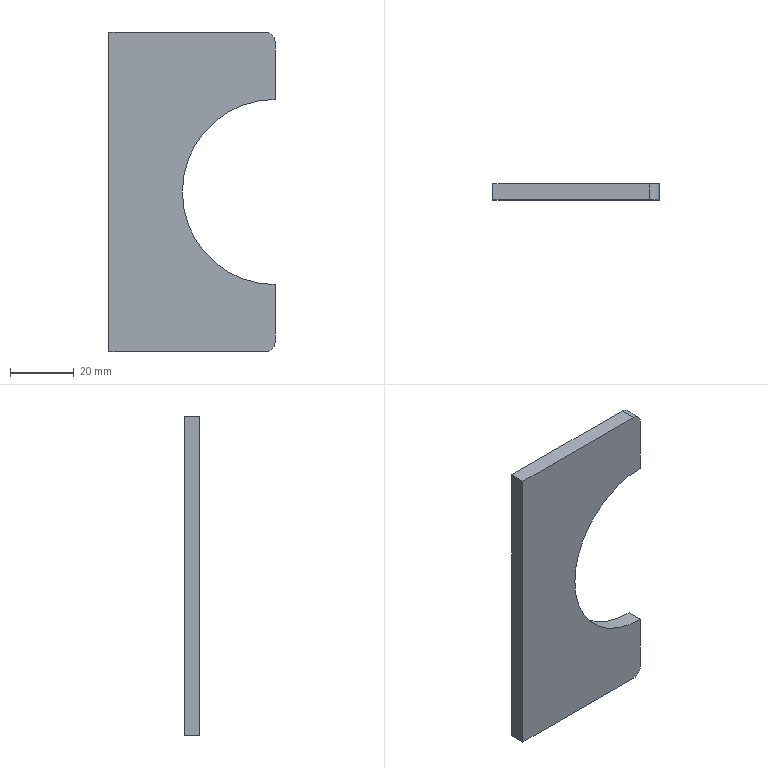Part | STEP file | JBJ-P-1004-03 | 1 solid | 10 faces | box 52 x 5 x 100 mm | volume 19375 mm3 | plane 7 | cylinder 3 | commonest cylinder face diameters 6 x2 58 x1
STEP:
#1=CARTESIAN_POINT('',(0.,0.,0.));
#2=VERTEX_POINT('',#1);
#3=CARTESIAN_POINT('',(0.,0.,100.));
#4=VERTEX_POINT('',#3);
#5=CARTESIAN_POINT('',(0.,0.,0.));
#6=DIRECTION('',(0.,0.,1.));
#7=VECTOR('',#6,1000.);
#8=LINE('',#5,#7);
#9=EDGE_CURVE('',#2,#4,#8,.T.);
#10=ORIENTED_EDGE('',*,*,#9,.T.);
#11=CARTESIAN_POINT('',(0.,5.,100.));
#12=VERTEX_POINT('',#11);
#13=CARTESIAN_POINT('',(0.,5.,100.));
#14=DIRECTION('',(0.,-1.,0.));
#15=VECTOR('',#14,1000.);
#16=LINE('',#13,#15);
#17=EDGE_CURVE('',#12,#4,#16,.T.);
#18=ORIENTED_EDGE('',*,*,#17,.F.);
#19=CARTESIAN_POINT('',(0.,5.,0.));
#20=VERTEX_POINT('',#19);
#21=CARTESIAN_POINT('',(0.,5.,0.));
#22=DIRECTION('',(0.,0.,1.));
#23=VECTOR('',#22,1000.);
#24=LINE('',#21,#23);
#25=EDGE_CURVE('',#20,#12,#24,.T.);
#26=ORIENTED_EDGE('',*,*,#25,.F.);
#27=CARTESIAN_POINT('',(0.,5.,0.));
#28=DIRECTION('',(0.,-1.,0.));
#29=VECTOR('',#28,1000.);
#30=LINE('',#27,#29);
#31=EDGE_CURVE('',#20,#2,#30,.T.);
#32=ORIENTED_EDGE('',*,*,#31,.T.);
#33=EDGE_LOOP('',(#10,#18,#26,#32));
#34=FACE_OUTER_BOUND('',#33,.T.);
#35=CARTESIAN_POINT('',(0.,5.,0.));
#36=DIRECTION('',(1.,0.,0.));
#37=DIRECTION('',(0.,0.,-1.));
#38=AXIS2_PLACEMENT_3D('',#35,#36,#37);
#39=PLANE('',#38);
#40=ADVANCED_FACE('',(#34),#39,.F.);
#41=CARTESIAN_POINT('',(49.,0.,100.));
#42=VERTEX_POINT('',#41);
#43=CARTESIAN_POINT('',(0.,0.,100.));
#44=DIRECTION('',(1.,0.,0.));
#45=VECTOR('',#44,1000.);
#46=LINE('',#43,#45);
#47=EDGE_CURVE('',#4,#42,#46,.T.);
#48=ORIENTED_EDGE('',*,*,#47,.T.);
#49=CARTESIAN_POINT('',(49.,5.,100.));
#50=VERTEX_POINT('',#49);
#51=CARTESIAN_POINT('',(49.,5.,100.));
#52=DIRECTION('',(0.,1.,0.));
#53=VECTOR('',#52,1000.);
#54=LINE('',#51,#53);
#55=EDGE_CURVE('',#42,#50,#54,.T.);
#56=ORIENTED_EDGE('',*,*,#55,.T.);
#57=CARTESIAN_POINT('',(0.,5.,100.));
#58=DIRECTION('',(1.,0.,0.));
#59=VECTOR('',#58,1000.);
#60=LINE('',#57,#59);
#61=EDGE_CURVE('',#12,#50,#60,.T.);
#62=ORIENTED_EDGE('',*,*,#61,.F.);
#63=ORIENTED_EDGE('',*,*,#17,.T.);
#64=EDGE_LOOP('',(#48,#56,#62,#63));
#65=FACE_OUTER_BOUND('',#64,.T.);
#66=CARTESIAN_POINT('',(0.,5.,100.));
#67=DIRECTION('',(0.,0.,-1.));
#68=DIRECTION('',(-1.,0.,0.));
#69=AXIS2_PLACEMENT_3D('',#66,#67,#68);
#70=PLANE('',#69);
#71=ADVANCED_FACE('',(#65),#70,.F.);
#72=CARTESIAN_POINT('',(52.,5.,97.));
#73=VERTEX_POINT('',#72);
#74=CARTESIAN_POINT('',(52.,5.,79.));
#75=VERTEX_POINT('',#74);
#76=CARTESIAN_POINT('',(52.,5.,79.));
#77=DIRECTION('',(0.,0.,-1.));
#78=VECTOR('',#77,1000.);
#79=LINE('',#76,#78);
#80=EDGE_CURVE('',#73,#75,#79,.T.);
#81=ORIENTED_EDGE('',*,*,#80,.F.);
#82=CARTESIAN_POINT('',(52.,0.,97.));
#83=VERTEX_POINT('',#82);
#84=CARTESIAN_POINT('',(52.,5.,97.));
#85=DIRECTION('',(0.,-1.,0.));
#86=VECTOR('',#85,1000.);
#87=LINE('',#84,#86);
#88=EDGE_CURVE('',#73,#83,#87,.T.);
#89=ORIENTED_EDGE('',*,*,#88,.T.);
#90=CARTESIAN_POINT('',(52.,0.,79.));
#91=VERTEX_POINT('',#90);
#92=CARTESIAN_POINT('',(52.,0.,79.));
#93=DIRECTION('',(0.,0.,-1.));
#94=VECTOR('',#93,1000.);
#95=LINE('',#92,#94);
#96=EDGE_CURVE('',#83,#91,#95,.T.);
#97=ORIENTED_EDGE('',*,*,#96,.T.);
#98=CARTESIAN_POINT('',(52.,5.,79.));
#99=DIRECTION('',(0.,-1.,0.));
#100=VECTOR('',#99,1000.);
#101=LINE('',#98,#100);
#102=EDGE_CURVE('',#75,#91,#101,.T.);
#103=ORIENTED_EDGE('',*,*,#102,.F.);
#104=EDGE_LOOP('',(#81,#89,#97,#103));
#105=FACE_OUTER_BOUND('',#104,.T.);
#106=CARTESIAN_POINT('',(52.,5.,79.));
#107=DIRECTION('',(-1.,0.,0.));
#108=DIRECTION('',(0.,0.,1.));
#109=AXIS2_PLACEMENT_3D('',#106,#107,#108);
#110=PLANE('',#109);
#111=ADVANCED_FACE('',(#105),#110,.F.);
#112=CARTESIAN_POINT('',(52.,0.,21.));
#113=VERTEX_POINT('',#112);
#114=CARTESIAN_POINT('',(52.,0.,50.));
#115=DIRECTION('',(0.,-1.,0.));
#116=DIRECTION('',(0.,0.,1.));
#117=AXIS2_PLACEMENT_3D('',#114,#115,#116);
#118=CIRCLE('',#117,29.);
#119=EDGE_CURVE('',#91,#113,#118,.T.);
#120=ORIENTED_EDGE('',*,*,#119,.T.);
#121=CARTESIAN_POINT('',(52.,5.,21.));
#122=VERTEX_POINT('',#121);
#123=CARTESIAN_POINT('',(52.,5.,21.));
#124=DIRECTION('',(0.,-1.,0.));
#125=VECTOR('',#124,1000.);
#126=LINE('',#123,#125);
#127=EDGE_CURVE('',#122,#113,#126,.T.);
#128=ORIENTED_EDGE('',*,*,#127,.F.);
#129=CARTESIAN_POINT('',(52.,5.,50.));
#130=DIRECTION('',(0.,-1.,0.));
#131=DIRECTION('',(0.,0.,1.));
#132=AXIS2_PLACEMENT_3D('',#129,#130,#131);
#133=CIRCLE('',#132,29.);
#134=EDGE_CURVE('',#75,#122,#133,.T.);
#135=ORIENTED_EDGE('',*,*,#134,.F.);
#136=ORIENTED_EDGE('',*,*,#102,.T.);
#137=EDGE_LOOP('',(#120,#128,#135,#136));
#138=FACE_OUTER_BOUND('',#137,.T.);
#139=CARTESIAN_POINT('',(52.,5.,50.));
#140=DIRECTION('',(0.,-1.,0.));
#141=DIRECTION('',(0.,0.,-1.));
#142=AXIS2_PLACEMENT_3D('',#139,#140,#141);
#143=CYLINDRICAL_SURFACE('',#142,29.);
#144=ADVANCED_FACE('',(#138),#143,.F.);
#145=CARTESIAN_POINT('',(52.,0.,3.));
#146=VERTEX_POINT('',#145);
#147=CARTESIAN_POINT('',(52.,0.,0.));
#148=DIRECTION('',(0.,0.,-1.));
#149=VECTOR('',#148,1000.);
#150=LINE('',#147,#149);
#151=EDGE_CURVE('',#113,#146,#150,.T.);
#152=ORIENTED_EDGE('',*,*,#151,.T.);
#153=CARTESIAN_POINT('',(52.,5.,3.));
#154=VERTEX_POINT('',#153);
#155=CARTESIAN_POINT('',(52.,5.,3.));
#156=DIRECTION('',(0.,1.,0.));
#157=VECTOR('',#156,1000.);
#158=LINE('',#155,#157);
#159=EDGE_CURVE('',#146,#154,#158,.T.);
#160=ORIENTED_EDGE('',*,*,#159,.T.);
#161=CARTESIAN_POINT('',(52.,5.,0.));
#162=DIRECTION('',(0.,0.,-1.));
#163=VECTOR('',#162,1000.);
#164=LINE('',#161,#163);
#165=EDGE_CURVE('',#122,#154,#164,.T.);
#166=ORIENTED_EDGE('',*,*,#165,.F.);
#167=ORIENTED_EDGE('',*,*,#127,.T.);
#168=EDGE_LOOP('',(#152,#160,#166,#167));
#169=FACE_OUTER_BOUND('',#168,.T.);
#170=CARTESIAN_POINT('',(52.,5.,0.));
#171=DIRECTION('',(-1.,0.,0.));
#172=DIRECTION('',(0.,0.,1.));
#173=AXIS2_PLACEMENT_3D('',#170,#171,#172);
#174=PLANE('',#173);
#175=ADVANCED_FACE('',(#169),#174,.F.);
#176=CARTESIAN_POINT('',(49.,5.,0.));
#177=VERTEX_POINT('',#176);
#178=CARTESIAN_POINT('',(0.,5.,0.));
#179=DIRECTION('',(-1.,0.,0.));
#180=VECTOR('',#179,1000.);
#181=LINE('',#178,#180);
#182=EDGE_CURVE('',#177,#20,#181,.T.);
#183=ORIENTED_EDGE('',*,*,#182,.F.);
#184=CARTESIAN_POINT('',(49.,0.,0.));
#185=VERTEX_POINT('',#184);
#186=CARTESIAN_POINT('',(49.,5.,0.));
#187=DIRECTION('',(0.,-1.,0.));
#188=VECTOR('',#187,1000.);
#189=LINE('',#186,#188);
#190=EDGE_CURVE('',#177,#185,#189,.T.);
#191=ORIENTED_EDGE('',*,*,#190,.T.);
#192=CARTESIAN_POINT('',(0.,0.,0.));
#193=DIRECTION('',(-1.,0.,0.));
#194=VECTOR('',#193,1000.);
#195=LINE('',#192,#194);
#196=EDGE_CURVE('',#185,#2,#195,.T.);
#197=ORIENTED_EDGE('',*,*,#196,.T.);
#198=ORIENTED_EDGE('',*,*,#31,.F.);
#199=EDGE_LOOP('',(#183,#191,#197,#198));
#200=FACE_OUTER_BOUND('',#199,.T.);
#201=CARTESIAN_POINT('',(0.,5.,0.));
#202=DIRECTION('',(0.,0.,1.));
#203=DIRECTION('',(1.,0.,0.));
#204=AXIS2_PLACEMENT_3D('',#201,#202,#203);
#205=PLANE('',#204);
#206=ADVANCED_FACE('',(#200),#205,.F.);
#207=ORIENTED_EDGE('',*,*,#61,.T.);
#208=CARTESIAN_POINT('',(49.,5.,97.));
#209=DIRECTION('',(0.,1.,0.));
#210=DIRECTION('',(0.,0.,1.));
#211=AXIS2_PLACEMENT_3D('',#208,#209,#210);
#212=CIRCLE('',#211,3.);
#213=EDGE_CURVE('',#50,#73,#212,.T.);
#214=ORIENTED_EDGE('',*,*,#213,.T.);
#215=ORIENTED_EDGE('',*,*,#80,.T.);
#216=ORIENTED_EDGE('',*,*,#134,.T.);
#217=ORIENTED_EDGE('',*,*,#165,.T.);
#218=CARTESIAN_POINT('',(49.,5.,3.));
#219=DIRECTION('',(0.,1.,0.));
#220=DIRECTION('',(0.,0.,1.));
#221=AXIS2_PLACEMENT_3D('',#218,#219,#220);
#222=CIRCLE('',#221,3.);
#223=EDGE_CURVE('',#154,#177,#222,.T.);
#224=ORIENTED_EDGE('',*,*,#223,.T.);
#225=ORIENTED_EDGE('',*,*,#182,.T.);
#226=ORIENTED_EDGE('',*,*,#25,.T.);
#227=EDGE_LOOP('',(#207,#214,#215,#216,#217,#224,#225,#226));
#228=FACE_OUTER_BOUND('',#227,.T.);
#229=CARTESIAN_POINT('',(52.,5.,50.));
#230=DIRECTION('',(0.,1.,0.));
#231=DIRECTION('',(0.,0.,1.));
#232=AXIS2_PLACEMENT_3D('',#229,#230,#231);
#233=PLANE('',#232);
#234=ADVANCED_FACE('',(#228),#233,.T.);
#235=ORIENTED_EDGE('',*,*,#96,.F.);
#236=CARTESIAN_POINT('',(49.,0.,97.));
#237=DIRECTION('',(0.,-1.,0.));
#238=DIRECTION('',(0.,0.,1.));
#239=AXIS2_PLACEMENT_3D('',#236,#237,#238);
#240=CIRCLE('',#239,3.);
#241=EDGE_CURVE('',#83,#42,#240,.T.);
#242=ORIENTED_EDGE('',*,*,#241,.T.);
#243=ORIENTED_EDGE('',*,*,#47,.F.);
#244=ORIENTED_EDGE('',*,*,#9,.F.);
#245=ORIENTED_EDGE('',*,*,#196,.F.);
#246=CARTESIAN_POINT('',(49.,0.,3.));
#247=DIRECTION('',(0.,-1.,0.));
#248=DIRECTION('',(0.,0.,1.));
#249=AXIS2_PLACEMENT_3D('',#246,#247,#248);
#250=CIRCLE('',#249,3.);
#251=EDGE_CURVE('',#185,#146,#250,.T.);
#252=ORIENTED_EDGE('',*,*,#251,.T.);
#253=ORIENTED_EDGE('',*,*,#151,.F.);
#254=ORIENTED_EDGE('',*,*,#119,.F.);
#255=EDGE_LOOP('',(#235,#242,#243,#244,#245,#252,#253,#254));
#256=FACE_OUTER_BOUND('',#255,.T.);
#257=CARTESIAN_POINT('',(52.,0.,50.));
#258=DIRECTION('',(0.,1.,0.));
#259=DIRECTION('',(0.,0.,1.));
#260=AXIS2_PLACEMENT_3D('',#257,#258,#259);
#261=PLANE('',#260);
#262=ADVANCED_FACE('',(#256),#261,.F.);
#263=ORIENTED_EDGE('',*,*,#213,.F.);
#264=ORIENTED_EDGE('',*,*,#55,.F.);
#265=ORIENTED_EDGE('',*,*,#241,.F.);
#266=ORIENTED_EDGE('',*,*,#88,.F.);
#267=EDGE_LOOP('',(#263,#264,#265,#266));
#268=FACE_OUTER_BOUND('',#267,.T.);
#269=CARTESIAN_POINT('',(49.,5.,97.));
#270=DIRECTION('',(0.,-1.,0.));
#271=DIRECTION('',(0.,0.,-1.));
#272=AXIS2_PLACEMENT_3D('',#269,#270,#271);
#273=CYLINDRICAL_SURFACE('',#272,3.);
#274=ADVANCED_FACE('',(#268),#273,.T.);
#275=ORIENTED_EDGE('',*,*,#223,.F.);
#276=ORIENTED_EDGE('',*,*,#159,.F.);
#277=ORIENTED_EDGE('',*,*,#251,.F.);
#278=ORIENTED_EDGE('',*,*,#190,.F.);
#279=EDGE_LOOP('',(#275,#276,#277,#278));
#280=FACE_OUTER_BOUND('',#279,.T.);
#281=CARTESIAN_POINT('',(49.,5.,3.));
#282=DIRECTION('',(0.,-1.,0.));
#283=DIRECTION('',(0.,0.,-1.));
#284=AXIS2_PLACEMENT_3D('',#281,#282,#283);
#285=CYLINDRICAL_SURFACE('',#284,3.);
#286=ADVANCED_FACE('',(#280),#285,.T.);
#287=CLOSED_SHELL('',(#40,#71,#111,#144,#175,#206,#234,#262,#274,#286));
#288=MANIFOLD_SOLID_BREP('',#287);
#289=CARTESIAN_POINT('',(0.,0.,0.));
#290=DIRECTION('',(0.,0.,1.));
#291=DIRECTION('',(1.,0.,0.));
#292=AXIS2_PLACEMENT_3D('',#289,#290,#291);
#293=(LENGTH_UNIT()NAMED_UNIT(*)SI_UNIT(.MILLI.,.METRE.));
#294=UNCERTAINTY_MEASURE_WITH_UNIT(LENGTH_MEASURE(0.00001),#293,'','');
#295=(NAMED_UNIT(*)PLANE_ANGLE_UNIT()SI_UNIT($,.RADIAN.));
#296=(NAMED_UNIT(*)SI_UNIT($,.STERADIAN.)SOLID_ANGLE_UNIT());
#297=(GEOMETRIC_REPRESENTATION_CONTEXT(3)GLOBAL_UNCERTAINTY_ASSIGNED_CONTEXT((#294))GLOBAL_UNIT_ASSIGNED_CONTEXT((#293,#295,#296))REPRESENTATION_CONTEXT('',''));
#298=ADVANCED_BREP_SHAPE_REPRESENTATION('',(#288,#292),#297);